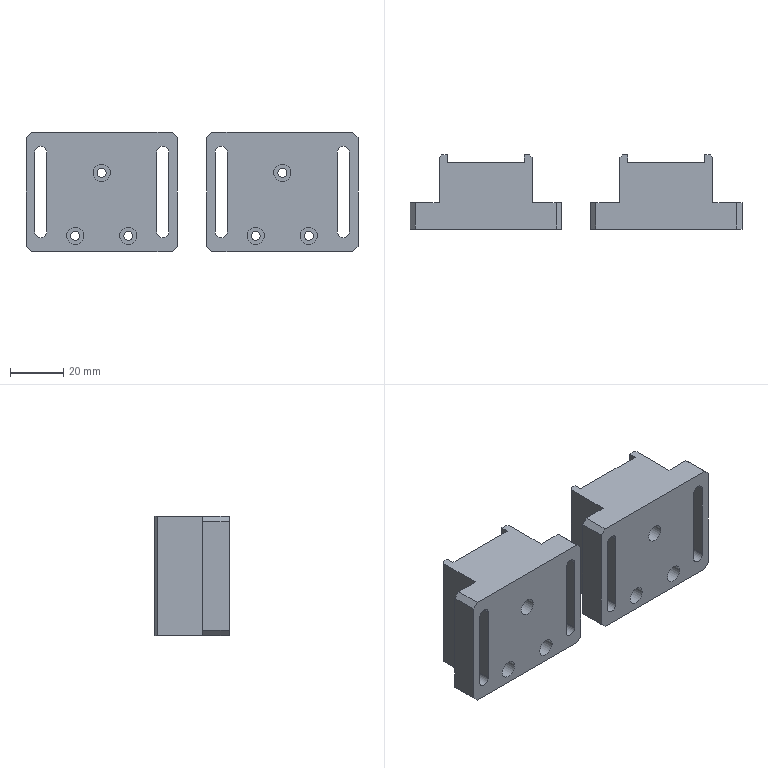Part | 2 solids | 74 faces | box 125 x 28 x 45 mm | volume 89629 mm3 | plane 54 | cylinder 20 | commonest cylinder face diameters 4.5 x8 3.4 x6 6.5 x6